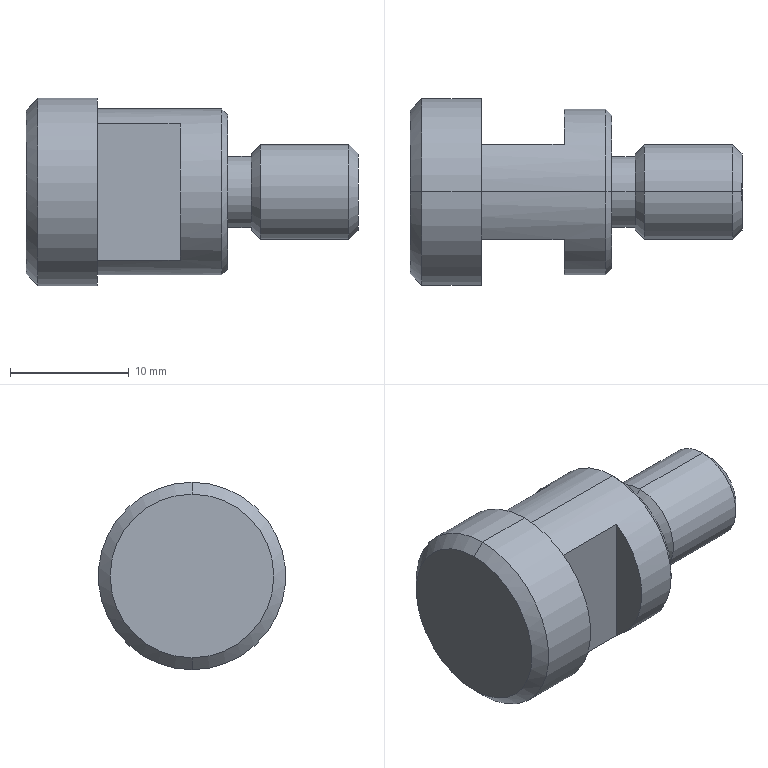Part | STEP file | _YU-03.stp | 1 solid | 25 faces | box 28 x 15.8 x 15.8 mm | volume 2997 mm3 | plane 9 | cone 8 | cylinder 8 | commonest cylinder face diameters 6 x2 8 x2 14 x2 15.8 x2